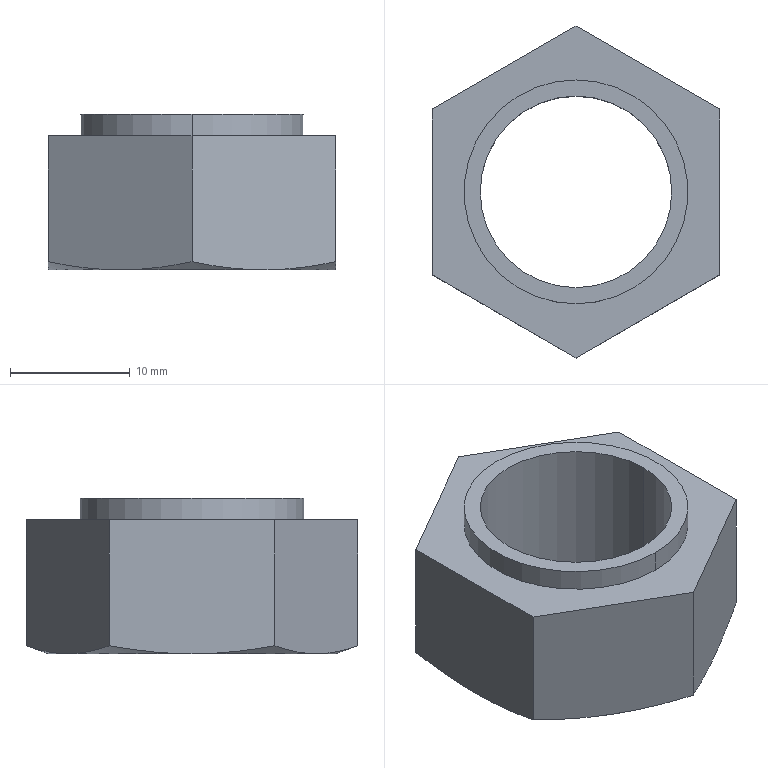Part | STEP file | 1 solid | 21 faces | box 24 x 27.713 x 13 mm | volume 3389 mm3 | plane 9 | cone 8 | cylinder 4 | commonest cylinder face diameters 16 x2 18.7 x2